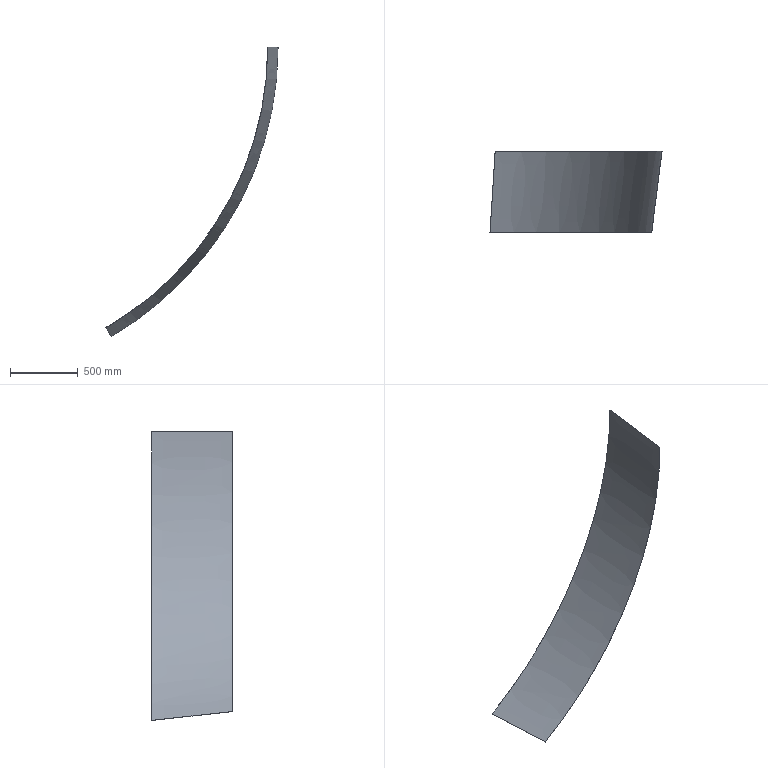Part | SolidWorks | features FlatPattern 1, ICE 1, LoftedBend 1, SheetMetal 1 | 1 solid | 6 faces | box 1273 x 598.126 x 2139 mm | volume 1534665 mm3 | spline 4 | plane 2